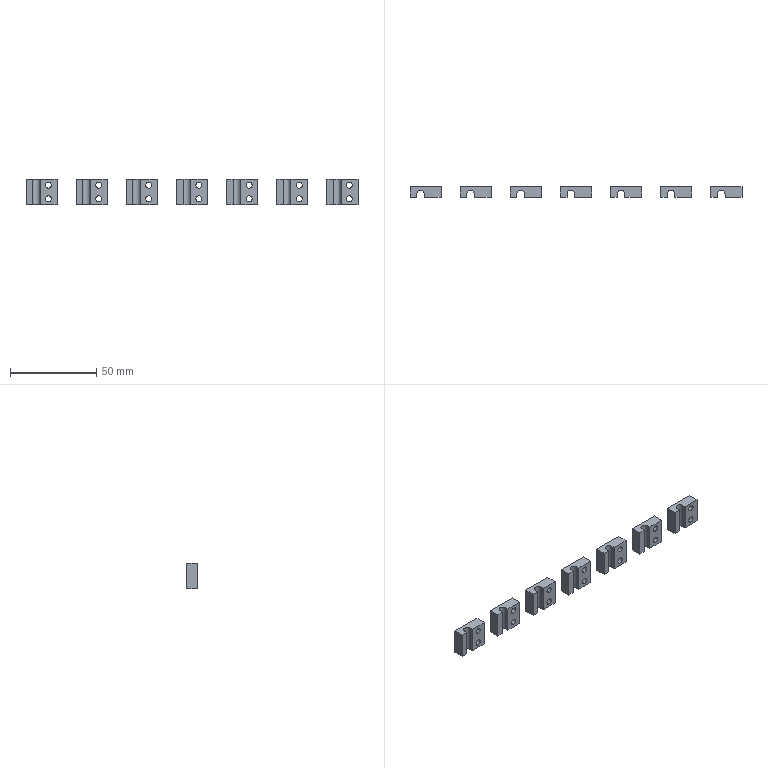CAM job | Mastercam | 3-axis milling, 5-axis milling, drilling | part box 192 x 6 x 15 mm | stock box 192 x 6 x 15 mm
Tools:
tool_number,name,type,diameter_mm,corner_radius_mm,flutes,flute_length_mm,overall_length_mm,shoulder_length_mm,holder_diameter_mm,length_offset,diameter_offset,default_rpm,default_feed_mm_min,default_plunge_mm_min,coolant
2,2 Flat End Mill,end mill,2,0,4,25,75,25,50,2,2,5000,600,600,COOL_OFF
5,3 Ball Mill / Bull Nose Mill,ball end mill,3,1.5,4,63,126,75.6,50,5,5,224595,63695.142,1000,COOL_OFF
7,4 Chamfer Mill,chamfer mill,4,0,4,25,75,30,50,7,7,6250,750,600,COOL_OFF
9,10 Flat End Mill,end mill,10,0,4,25,75,25,50,9,9,1000,120,600,COOL_OFF
10,10 Flat End Mill,end mill,10,0,4,25,75,25,50,10,10,1000,120,600,COOL_OFF
20,63 Flat End Mill,end mill,63,0,4,25,75,25,50,20,20,159,19.08,600,COOL_OFF
Operations:
seq,operation,operation_type,tool_number,tool_name,tool_diameter_mm,spindle_rpm,feed_mm_min,plunge_mm_min,retract_mm_min,cycle_time_s,wcs,posted,nc_file
1,Facing - [WCS: Plane] - [Tplane: Plane],Facing,20,63 Flat End Mill,63,4000,1000,600,1200,18.238,Plane,yes,.nc
2,Contour (Ramp) - [WCS: Plane] - [Tplane: Plane],Contour,9,10 Flat End Mill,10,10000,4000,600,1200,149.803,Plane,yes,.nc
3,Contour (2D) - [WCS: Plane] - [Tplane: Plane],Contour,10,10 Flat End Mill,10,8000,1000,600,1200,52.919,Plane,yes,.nc
4,3D High Speed (Area roughing) - [WCS: Plane] - [Tplane: Plane],HighSpeed3D,2,2 Flat End Mill,2,7000,3000,600,1200,24.54,Plane,yes,.nc
5,Contour (2D) - [WCS: Plane] - [Tplane: Plane],Contour,2,2 Flat End Mill,2,8000,1000,600,1200,3.808,Plane,yes,.nc
6,Surface Finish Flowline - [WCS: Plane] - [Tplane: Plane],MultiSurfaceFinishFlowline,5,3 Ball Mill / Bull Nose Mill,3,7000,3000,1000,2000,25.082,Plane,yes,.nc
7,Deburr 5-axis - [WCS: Plane] - [Tplane: Plane],459,5,3 Ball Mill / Bull Nose Mill,3,7000,1000,1000,2000,11.096,Plane,yes,.nc
8,Drill/Counterbore - [WCS: Plane] - [Tplane: Plane],Drill,7,4 Chamfer Mill,4,6000,200,600,1200,1.977,Plane,yes,.nc
9,Transform/Translate Rectangular/Coordinate/NCI,XForm,,,,0,0,0,0,399.016,Plane,yes,.nc
10,Facing - [WCS: Plane] - [Tplane: Plane],Facing,20,63 Flat End Mill,63,4000,2000,600,1200,231.827,Plane,yes,.nc